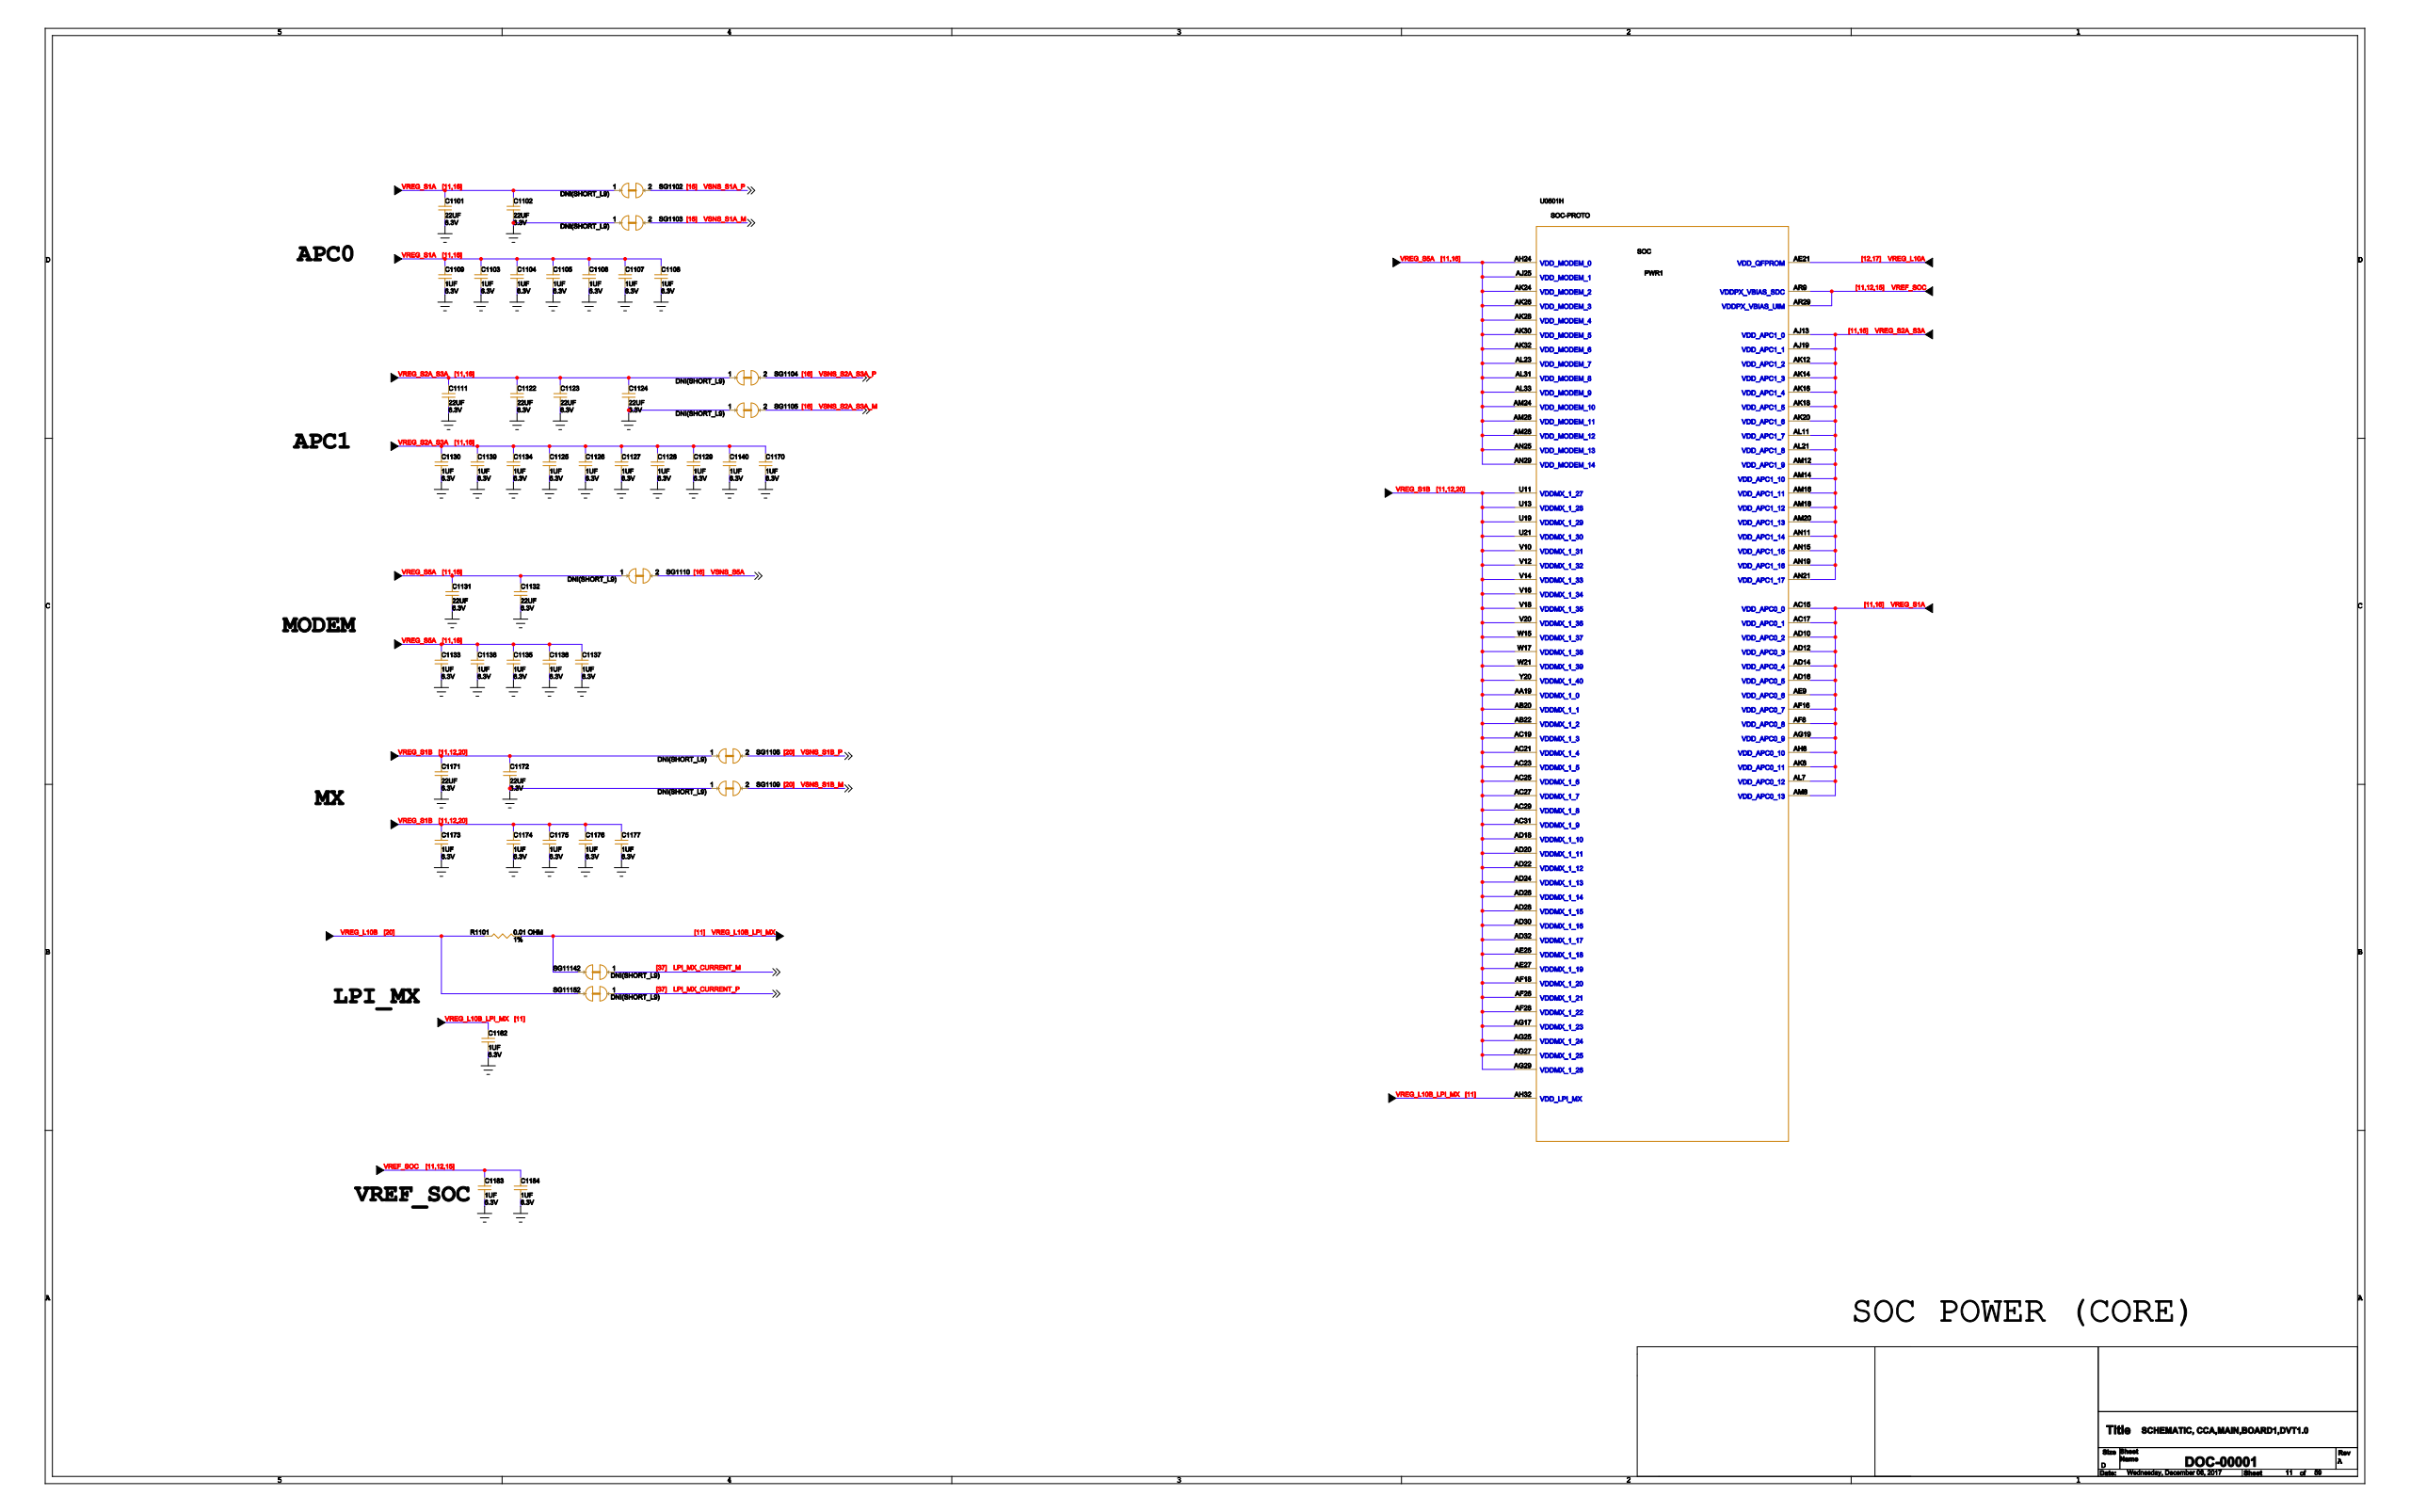Circuit board | KiCad | 1657 parts | 1365 nets | one sheet of the schematic
Parts on this sheet (reference | value | footprint):
C1101
C1102
C1103
C1104
C1105
C1106
C1107
C1108
C1109
C1111
C1122
C1123
C1124
C1125
C1126
C1127
C1128
C1129
C1130
C1131
C1132
C1133
C1134
C1135
C1136
C1137
C1138
C1139
C1140
C1170
C1171
C1172
C1173
C1174
C1175
C1176
C1177
C1182
C1183
C1184
R1101
SG1102
SG1103
SG1104
SG1105
SG1108
SG1109
SG1110
SG1114
SG1115
U0501
Nets of these parts (net: part-pin ...):
GND: C1101-2 C1102-2 C1103-2 C1104-2 C1105-2 C1106-2 C1107-2 C1108-2 C1109-2 C1111-2 C1122-2 C1123-2 C1124-2 C1125-2 C1126-2 C1127-2 C1128-2 C1129-2 C1130-2 C1131-2 C1132-2 C1133-2 C1134-2 C1135-2 C1136-2 C1137-2 C1138-2 C1139-2 C1140-2 C1170-2 C1171-2 C1172-2 C1173-2 C1174-2 C1175-2 C1176-2 C1177-2 C1182-2 C1183-2 C1184-2 SG1103-1 SG1105-1 SG1109-1
VREG_S1A: C1101-1 C1102-1 C1103-1 C1104-1 C1105-1 C1106-1 C1107-1 C1108-1 C1109-1 SG1102-1 U0501-AC15 U0501-AC17 U0501-AD10 U0501-AD12 U0501-AD14 U0501-AD16 U0501-AE9 U0501-AF8 U0501-AF16 U0501-AG19 U0501-AH8 U0501-AK8 U0501-AL7 U0501-AM8
VREG_S2A_S3A: C1111-1 C1122-1 C1123-1 C1124-1 C1125-1 C1126-1 C1127-1 C1128-1 C1129-1 C1130-1 C1134-1 C1139-1 C1140-1 C1170-1 SG1104-1 U0501-AJ13 U0501-AJ19 U0501-AK12 U0501-AK14 U0501-AK16 U0501-AK18 U0501-AK20 U0501-AL11 U0501-AL21 U0501-AM12 U0501-AM14 U0501-AM16 U0501-AM18 U0501-AM20 U0501-AN11 U0501-AN15 U0501-AN19 U0501-AN21
VSNS_S1B_M: SG1109-2
I_MX_CURRENT_P: SG1115-1
VREG_L10B: R1101-2 SG1115-2
VREG_S5A: C1131-1 C1132-1 C1133-1 C1135-1 C1136-1 C1137-1 C1138-1 SG1110-1 U0501-AH24 U0501-AJ25 U0501-AK24 U0501-AK26 U0501-AK28 U0501-AK30 U0501-AK32 U0501-AL23 U0501-AL31 U0501-AL33 U0501-AM24 U0501-AM26 U0501-AM28 U0501-AN25 U0501-AN29
VSNS_S5A: SG1110-2
VSNS_S2A_S3A_M: SG1105-2
VSNS_S2A_S3A_P: SG1104-2
VREG_S1B: C1171-1 C1172-1 C1173-1 C1174-1 C1175-1 C1176-1 C1177-1 SG1108-1 U0501-AA19 U0501-AB20 U0501-AB22 U0501-AC19 U0501-AC21 U0501-AC23 U0501-AC25 U0501-AC27 U0501-AC29 U0501-AC31 U0501-AD18 U0501-AD20 U0501-AD22 U0501-AD24 U0501-AD26 U0501-AD28 U0501-AD30 U0501-AD32 U0501-AE25 U0501-AE27 U0501-AF18 U0501-AF26 U0501-AF28 U0501-AG17 U0501-AG25 U0501-AG27 U0501-AG29 U0501-U11 U0501-U13 U0501-U19 U0501-U21 U0501-V10 U0501-V12 U0501-V14 U0501-V16 U0501-V18 U0501-V20 U0501-W15 U0501-W17 U0501-W21 U0501-Y20
VREG_L10A: U0501-AE21
VREF_SOC: C1183-1 C1184-1 U0501-AR9 U0501-AR29
EG_L10B_LPI_MX: C1182-1 R1101-1 SG1114-2 U0501-AH32
I_MX_CURRENT_M: SG1114-1
VSNS_S1B_P: SG1108-2
VSNS_S1A_M: SG1103-2
VSNS_S1A_P: SG1102-2